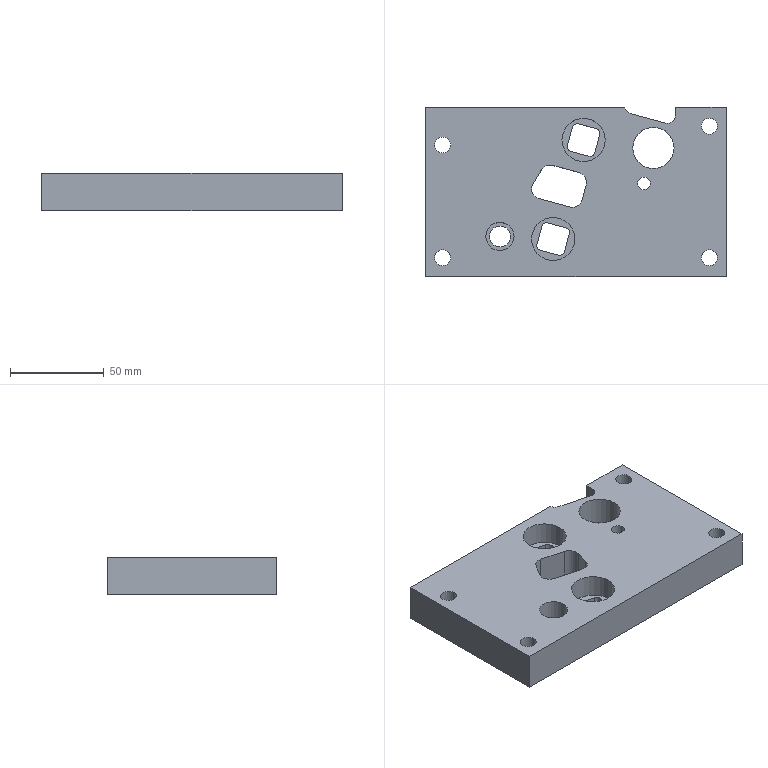Part | NX | features solid 2 | 1 solid | 67 faces | box 160 x 90 x 20 mm | volume 238632 mm3 | cylinder 34 | plane 33 | commonest cylinder face diameters 5.15 x8 6 x4 8.5 x4 11 x4 14 x4 4 x2